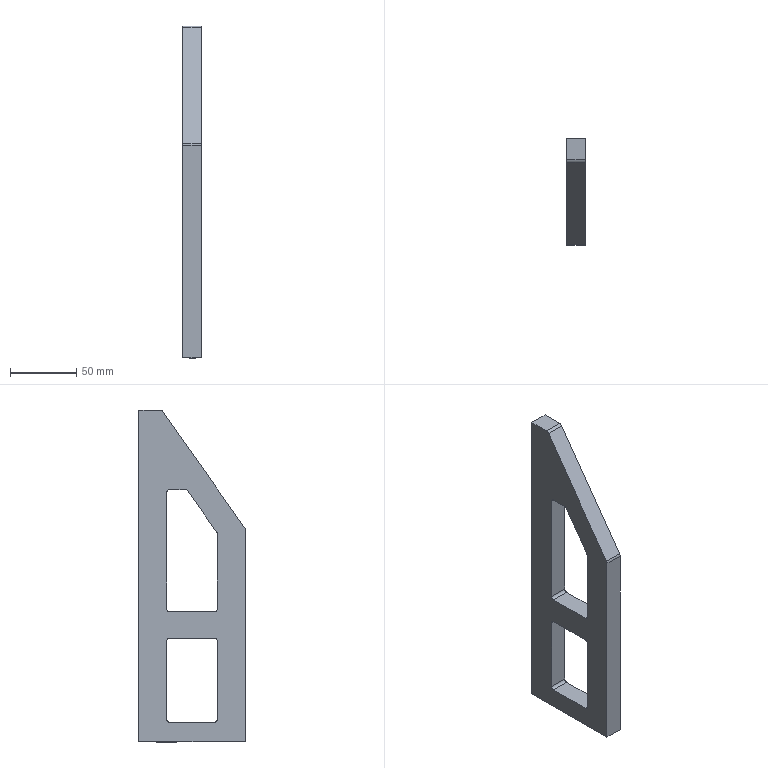Part | SolidWorks | features Fillet 3, Cut 2, HoleWzd 2, Extrusion 1 | 1 solid | 47 faces | box 14 x 80 x 250 mm | volume 162900 mm3 | cylinder 21 | plane 16 | cone 10 | commonest cylinder face diameters 4 x9 3.3 x6 4.2 x4 6 x2
STEP:
#1=CARTESIAN_POINT('',(50.,192.243,112.35));
#2=VERTEX_POINT('',#1);
#3=CARTESIAN_POINT('',(50.,192.243,115.65));
#4=VERTEX_POINT('',#3);
#5=CARTESIAN_POINT('',(50.,192.243,114.));
#6=DIRECTION('',(0.,1.,0.));
#7=DIRECTION('',(0.,0.,1.));
#8=AXIS2_PLACEMENT_3D('',#5,#6,#7);
#9=CIRCLE('',#8,1.65);
#10=EDGE_CURVE('',#2,#4,#9,.T.);
#11=ORIENTED_EDGE('',*,*,#10,.F.);
#12=CARTESIAN_POINT('',(50.,203.743,112.35));
#13=VERTEX_POINT('',#12);
#14=CARTESIAN_POINT('',(50.,203.743,112.35));
#15=DIRECTION('',(0.,1.,0.));
#16=VECTOR('',#15,1000.);
#17=LINE('',#14,#16);
#18=EDGE_CURVE('',#2,#13,#17,.T.);
#19=ORIENTED_EDGE('',*,*,#18,.T.);
#20=CARTESIAN_POINT('',(50.,203.743,115.65));
#21=VERTEX_POINT('',#20);
#22=CARTESIAN_POINT('',(50.,203.743,114.));
#23=DIRECTION('',(0.,1.,0.));
#24=DIRECTION('',(0.,0.,1.));
#25=AXIS2_PLACEMENT_3D('',#22,#23,#24);
#26=CIRCLE('',#25,1.65);
#27=EDGE_CURVE('',#13,#21,#26,.T.);
#28=ORIENTED_EDGE('',*,*,#27,.T.);
#29=CARTESIAN_POINT('',(50.,203.743,115.65));
#30=DIRECTION('',(0.,1.,0.));
#31=VECTOR('',#30,1000.);
#32=LINE('',#29,#31);
#33=EDGE_CURVE('',#4,#21,#32,.T.);
#34=ORIENTED_EDGE('',*,*,#33,.F.);
#35=EDGE_LOOP('',(#11,#19,#28,#34));
#36=FACE_OUTER_BOUND('',#35,.T.);
#37=CARTESIAN_POINT('',(50.,203.743,114.));
#38=DIRECTION('',(0.,1.,0.));
#39=DIRECTION('',(0.,0.,1.));
#40=AXIS2_PLACEMENT_3D('',#37,#38,#39);
#41=CYLINDRICAL_SURFACE('',#40,1.65);
#42=ADVANCED_FACE('',(#36),#41,.F.);
#43=CARTESIAN_POINT('',(50.,191.252,114.));
#44=VERTEX_POINT('',#43);
#45=CARTESIAN_POINT('',(50.,192.243,115.65));
#46=DIRECTION('',(0.,0.515,0.8572));
#47=VECTOR('',#46,1000.);
#48=LINE('',#45,#47);
#49=EDGE_CURVE('',#44,#4,#48,.T.);
#50=ORIENTED_EDGE('',*,*,#49,.F.);
#51=CARTESIAN_POINT('',(50.,192.243,112.35));
#52=DIRECTION('',(0.,0.515,-0.8572));
#53=VECTOR('',#52,1000.);
#54=LINE('',#51,#53);
#55=EDGE_CURVE('',#44,#2,#54,.T.);
#56=ORIENTED_EDGE('',*,*,#55,.T.);
#57=ORIENTED_EDGE('',*,*,#10,.T.);
#58=EDGE_LOOP('',(#50,#56,#57));
#59=FACE_OUTER_BOUND('',#58,.T.);
#60=CARTESIAN_POINT('',(50.,192.243,114.));
#61=DIRECTION('',(0.,1.,0.));
#62=DIRECTION('',(0.,0.,1.));
#63=AXIS2_PLACEMENT_3D('',#60,#61,#62);
#64=CONICAL_SURFACE('',#63,1.65,1.03);
#65=ADVANCED_FACE('',(#59),#64,.F.);
#66=CARTESIAN_POINT('',(50.,192.243,172.35));
#67=VERTEX_POINT('',#66);
#68=CARTESIAN_POINT('',(50.,192.243,175.65));
#69=VERTEX_POINT('',#68);
#70=CARTESIAN_POINT('',(50.,192.243,174.));
#71=DIRECTION('',(0.,1.,0.));
#72=DIRECTION('',(0.,0.,1.));
#73=AXIS2_PLACEMENT_3D('',#70,#71,#72);
#74=CIRCLE('',#73,1.65);
#75=EDGE_CURVE('',#67,#69,#74,.T.);
#76=ORIENTED_EDGE('',*,*,#75,.F.);
#77=CARTESIAN_POINT('',(50.,203.743,172.35));
#78=VERTEX_POINT('',#77);
#79=CARTESIAN_POINT('',(50.,203.743,172.35));
#80=DIRECTION('',(0.,1.,0.));
#81=VECTOR('',#80,1000.);
#82=LINE('',#79,#81);
#83=EDGE_CURVE('',#67,#78,#82,.T.);
#84=ORIENTED_EDGE('',*,*,#83,.T.);
#85=CARTESIAN_POINT('',(50.,203.743,175.65));
#86=VERTEX_POINT('',#85);
#87=CARTESIAN_POINT('',(50.,203.743,174.));
#88=DIRECTION('',(0.,1.,0.));
#89=DIRECTION('',(0.,0.,1.));
#90=AXIS2_PLACEMENT_3D('',#87,#88,#89);
#91=CIRCLE('',#90,1.65);
#92=EDGE_CURVE('',#78,#86,#91,.T.);
#93=ORIENTED_EDGE('',*,*,#92,.T.);
#94=CARTESIAN_POINT('',(50.,203.743,175.65));
#95=DIRECTION('',(0.,1.,0.));
#96=VECTOR('',#95,1000.);
#97=LINE('',#94,#96);
#98=EDGE_CURVE('',#69,#86,#97,.T.);
#99=ORIENTED_EDGE('',*,*,#98,.F.);
#100=EDGE_LOOP('',(#76,#84,#93,#99));
#101=FACE_OUTER_BOUND('',#100,.T.);
#102=CARTESIAN_POINT('',(50.,203.743,174.));
#103=DIRECTION('',(0.,1.,0.));
#104=DIRECTION('',(0.,0.,1.));
#105=AXIS2_PLACEMENT_3D('',#102,#103,#104);
#106=CYLINDRICAL_SURFACE('',#105,1.65);
#107=ADVANCED_FACE('',(#101),#106,.F.);
#108=CARTESIAN_POINT('',(50.,191.252,174.));
#109=VERTEX_POINT('',#108);
#110=CARTESIAN_POINT('',(50.,192.243,175.65));
#111=DIRECTION('',(0.,0.515,0.8572));
#112=VECTOR('',#111,1000.);
#113=LINE('',#110,#112);
#114=EDGE_CURVE('',#109,#69,#113,.T.);
#115=ORIENTED_EDGE('',*,*,#114,.F.);
#116=CARTESIAN_POINT('',(50.,192.243,172.35));
#117=DIRECTION('',(0.,0.515,-0.8572));
#118=VECTOR('',#117,1000.);
#119=LINE('',#116,#118);
#120=EDGE_CURVE('',#109,#67,#119,.T.);
#121=ORIENTED_EDGE('',*,*,#120,.T.);
#122=ORIENTED_EDGE('',*,*,#75,.T.);
#123=EDGE_LOOP('',(#115,#121,#122));
#124=FACE_OUTER_BOUND('',#123,.T.);
#125=CARTESIAN_POINT('',(50.,192.243,174.));
#126=DIRECTION('',(0.,1.,0.));
#127=DIRECTION('',(0.,0.,1.));
#128=AXIS2_PLACEMENT_3D('',#125,#126,#127);
#129=CONICAL_SURFACE('',#128,1.65,1.03);
#130=ADVANCED_FACE('',(#124),#129,.F.);
#131=CARTESIAN_POINT('',(50.,192.243,232.35));
#132=VERTEX_POINT('',#131);
#133=CARTESIAN_POINT('',(50.,192.243,235.65));
#134=VERTEX_POINT('',#133);
#135=CARTESIAN_POINT('',(50.,192.243,234.));
#136=DIRECTION('',(0.,1.,0.));
#137=DIRECTION('',(0.,0.,1.));
#138=AXIS2_PLACEMENT_3D('',#135,#136,#137);
#139=CIRCLE('',#138,1.65);
#140=EDGE_CURVE('',#132,#134,#139,.T.);
#141=ORIENTED_EDGE('',*,*,#140,.F.);
#142=CARTESIAN_POINT('',(50.,203.743,232.35));
#143=VERTEX_POINT('',#142);
#144=CARTESIAN_POINT('',(50.,203.743,232.35));
#145=DIRECTION('',(0.,1.,0.));
#146=VECTOR('',#145,1000.);
#147=LINE('',#144,#146);
#148=EDGE_CURVE('',#132,#143,#147,.T.);
#149=ORIENTED_EDGE('',*,*,#148,.T.);
#150=CARTESIAN_POINT('',(50.,203.743,235.65));
#151=VERTEX_POINT('',#150);
#152=CARTESIAN_POINT('',(50.,203.743,234.));
#153=DIRECTION('',(0.,1.,0.));
#154=DIRECTION('',(0.,0.,1.));
#155=AXIS2_PLACEMENT_3D('',#152,#153,#154);
#156=CIRCLE('',#155,1.65);
#157=EDGE_CURVE('',#143,#151,#156,.T.);
#158=ORIENTED_EDGE('',*,*,#157,.T.);
#159=CARTESIAN_POINT('',(50.,203.743,235.65));
#160=DIRECTION('',(0.,1.,0.));
#161=VECTOR('',#160,1000.);
#162=LINE('',#159,#161);
#163=EDGE_CURVE('',#134,#151,#162,.T.);
#164=ORIENTED_EDGE('',*,*,#163,.F.);
#165=EDGE_LOOP('',(#141,#149,#158,#164));
#166=FACE_OUTER_BOUND('',#165,.T.);
#167=CARTESIAN_POINT('',(50.,203.743,234.));
#168=DIRECTION('',(0.,1.,0.));
#169=DIRECTION('',(0.,0.,1.));
#170=AXIS2_PLACEMENT_3D('',#167,#168,#169);
#171=CYLINDRICAL_SURFACE('',#170,1.65);
#172=ADVANCED_FACE('',(#166),#171,.F.);
#173=CARTESIAN_POINT('',(50.,191.252,234.));
#174=VERTEX_POINT('',#173);
#175=CARTESIAN_POINT('',(50.,192.243,235.65));
#176=DIRECTION('',(0.,0.515,0.8572));
#177=VECTOR('',#176,1000.);
#178=LINE('',#175,#177);
#179=EDGE_CURVE('',#174,#134,#178,.T.);
#180=ORIENTED_EDGE('',*,*,#179,.F.);
#181=CARTESIAN_POINT('',(50.,192.243,232.35));
#182=DIRECTION('',(0.,0.515,-0.8572));
#183=VECTOR('',#182,1000.);
#184=LINE('',#181,#183);
#185=EDGE_CURVE('',#174,#132,#184,.T.);
#186=ORIENTED_EDGE('',*,*,#185,.T.);
#187=ORIENTED_EDGE('',*,*,#140,.T.);
#188=EDGE_LOOP('',(#180,#186,#187));
#189=FACE_OUTER_BOUND('',#188,.T.);
#190=CARTESIAN_POINT('',(50.,192.243,234.));
#191=DIRECTION('',(0.,1.,0.));
#192=DIRECTION('',(0.,0.,1.));
#193=AXIS2_PLACEMENT_3D('',#190,#191,#192);
#194=CONICAL_SURFACE('',#193,1.65,1.03);
#195=ADVANCED_FACE('',(#189),#194,.F.);
#196=CARTESIAN_POINT('',(50.5,186.643,14.));
#197=VERTEX_POINT('',#196);
#198=CARTESIAN_POINT('',(50.5,190.843,14.));
#199=VERTEX_POINT('',#198);
#200=CARTESIAN_POINT('',(50.5,188.743,14.));
#201=DIRECTION('',(0.,0.,-1.));
#202=DIRECTION('',(0.,1.,0.));
#203=AXIS2_PLACEMENT_3D('',#200,#201,#202);
#204=CIRCLE('',#203,2.1);
#205=EDGE_CURVE('',#197,#199,#204,.T.);
#206=ORIENTED_EDGE('',*,*,#205,.F.);
#207=CARTESIAN_POINT('',(50.5,186.643,0.));
#208=VERTEX_POINT('',#207);
#209=CARTESIAN_POINT('',(50.5,186.643,0.));
#210=DIRECTION('',(0.,0.,-1.));
#211=VECTOR('',#210,1000.);
#212=LINE('',#209,#211);
#213=EDGE_CURVE('',#197,#208,#212,.T.);
#214=ORIENTED_EDGE('',*,*,#213,.T.);
#215=CARTESIAN_POINT('',(50.5,190.843,0.));
#216=VERTEX_POINT('',#215);
#217=CARTESIAN_POINT('',(50.5,188.743,0.));
#218=DIRECTION('',(0.,0.,-1.));
#219=DIRECTION('',(0.,1.,0.));
#220=AXIS2_PLACEMENT_3D('',#217,#218,#219);
#221=CIRCLE('',#220,2.1);
#222=EDGE_CURVE('',#208,#216,#221,.T.);
#223=ORIENTED_EDGE('',*,*,#222,.T.);
#224=CARTESIAN_POINT('',(50.5,190.843,0.));
#225=DIRECTION('',(0.,0.,-1.));
#226=VECTOR('',#225,1000.);
#227=LINE('',#224,#226);
#228=EDGE_CURVE('',#199,#216,#227,.T.);
#229=ORIENTED_EDGE('',*,*,#228,.F.);
#230=EDGE_LOOP('',(#206,#214,#223,#229));
#231=FACE_OUTER_BOUND('',#230,.T.);
#232=CARTESIAN_POINT('',(50.5,188.743,0.));
#233=DIRECTION('',(0.,0.,-1.));
#234=DIRECTION('',(0.,1.,0.));
#235=AXIS2_PLACEMENT_3D('',#232,#233,#234);
#236=CYLINDRICAL_SURFACE('',#235,2.1);
#237=ADVANCED_FACE('',(#231),#236,.F.);
#238=CARTESIAN_POINT('',(50.5,188.743,15.262));
#239=VERTEX_POINT('',#238);
#240=CARTESIAN_POINT('',(50.5,190.843,14.));
#241=DIRECTION('',(0.,0.8572,-0.515));
#242=VECTOR('',#241,1000.);
#243=LINE('',#240,#242);
#244=EDGE_CURVE('',#239,#199,#243,.T.);
#245=ORIENTED_EDGE('',*,*,#244,.F.);
#246=CARTESIAN_POINT('',(50.5,186.643,14.));
#247=DIRECTION('',(0.,-0.8572,-0.515));
#248=VECTOR('',#247,1000.);
#249=LINE('',#246,#248);
#250=EDGE_CURVE('',#239,#197,#249,.T.);
#251=ORIENTED_EDGE('',*,*,#250,.T.);
#252=ORIENTED_EDGE('',*,*,#205,.T.);
#253=EDGE_LOOP('',(#245,#251,#252));
#254=FACE_OUTER_BOUND('',#253,.T.);
#255=CARTESIAN_POINT('',(50.5,188.743,14.));
#256=DIRECTION('',(0.,0.,-1.));
#257=DIRECTION('',(0.,1.,0.));
#258=AXIS2_PLACEMENT_3D('',#255,#256,#257);
#259=CONICAL_SURFACE('',#258,2.1,1.03);
#260=ADVANCED_FACE('',(#254),#259,.F.);
#261=CARTESIAN_POINT('',(50.,136.645,14.));
#262=VERTEX_POINT('',#261);
#263=CARTESIAN_POINT('',(50.,140.845,14.));
#264=VERTEX_POINT('',#263);
#265=CARTESIAN_POINT('',(50.,138.745,14.));
#266=DIRECTION('',(0.,0.,-1.));
#267=DIRECTION('',(0.,1.,0.));
#268=AXIS2_PLACEMENT_3D('',#265,#266,#267);
#269=CIRCLE('',#268,2.1);
#270=EDGE_CURVE('',#262,#264,#269,.T.);
#271=ORIENTED_EDGE('',*,*,#270,.F.);
#272=CARTESIAN_POINT('',(50.,136.645,0.));
#273=VERTEX_POINT('',#272);
#274=CARTESIAN_POINT('',(50.,136.645,0.));
#275=DIRECTION('',(0.,0.,-1.));
#276=VECTOR('',#275,1000.);
#277=LINE('',#274,#276);
#278=EDGE_CURVE('',#262,#273,#277,.T.);
#279=ORIENTED_EDGE('',*,*,#278,.T.);
#280=CARTESIAN_POINT('',(50.,140.845,0.));
#281=VERTEX_POINT('',#280);
#282=CARTESIAN_POINT('',(50.,138.745,0.));
#283=DIRECTION('',(0.,0.,-1.));
#284=DIRECTION('',(0.,1.,0.));
#285=AXIS2_PLACEMENT_3D('',#282,#283,#284);
#286=CIRCLE('',#285,2.1);
#287=EDGE_CURVE('',#273,#281,#286,.T.);
#288=ORIENTED_EDGE('',*,*,#287,.T.);
#289=CARTESIAN_POINT('',(50.,140.845,0.));
#290=DIRECTION('',(0.,0.,-1.));
#291=VECTOR('',#290,1000.);
#292=LINE('',#289,#291);
#293=EDGE_CURVE('',#264,#281,#292,.T.);
#294=ORIENTED_EDGE('',*,*,#293,.F.);
#295=EDGE_LOOP('',(#271,#279,#288,#294));
#296=FACE_OUTER_BOUND('',#295,.T.);
#297=CARTESIAN_POINT('',(50.,138.745,0.));
#298=DIRECTION('',(0.,0.,-1.));
#299=DIRECTION('',(0.,1.,0.));
#300=AXIS2_PLACEMENT_3D('',#297,#298,#299);
#301=CYLINDRICAL_SURFACE('',#300,2.1);
#302=ADVANCED_FACE('',(#296),#301,.F.);
#303=CARTESIAN_POINT('',(50.,138.745,15.262));
#304=VERTEX_POINT('',#303);
#305=CARTESIAN_POINT('',(50.,140.845,14.));
#306=DIRECTION('',(0.,0.8572,-0.515));
#307=VECTOR('',#306,1000.);
#308=LINE('',#305,#307);
#309=EDGE_CURVE('',#304,#264,#308,.T.);
#310=ORIENTED_EDGE('',*,*,#309,.F.);
#311=CARTESIAN_POINT('',(50.,136.645,14.));
#312=DIRECTION('',(0.,-0.8572,-0.515));
#313=VECTOR('',#312,1000.);
#314=LINE('',#311,#313);
#315=EDGE_CURVE('',#304,#262,#314,.T.);
#316=ORIENTED_EDGE('',*,*,#315,.T.);
#317=ORIENTED_EDGE('',*,*,#270,.T.);
#318=EDGE_LOOP('',(#310,#316,#317));
#319=FACE_OUTER_BOUND('',#318,.T.);
#320=CARTESIAN_POINT('',(50.,138.745,14.));
#321=DIRECTION('',(0.,0.,-1.));
#322=DIRECTION('',(0.,1.,0.));
#323=AXIS2_PLACEMENT_3D('',#320,#321,#322);
#324=CONICAL_SURFACE('',#323,2.1,1.03);
#325=ADVANCED_FACE('',(#319),#324,.F.);
#326=CARTESIAN_POINT('',(50.,203.743,114.));
#327=DIRECTION('',(0.,1.,0.));
#328=DIRECTION('',(0.,0.,1.));
#329=AXIS2_PLACEMENT_3D('',#326,#327,#328);
#330=CIRCLE('',#329,1.65);
#331=EDGE_CURVE('',#21,#13,#330,.T.);
#332=ORIENTED_EDGE('',*,*,#331,.F.);
#333=ORIENTED_EDGE('',*,*,#27,.F.);
#334=EDGE_LOOP('',(#332,#333));
#335=FACE_BOUND('',#334,.T.);
#336=CARTESIAN_POINT('',(50.,203.743,174.));
#337=DIRECTION('',(0.,1.,0.));
#338=DIRECTION('',(0.,0.,1.));
#339=AXIS2_PLACEMENT_3D('',#336,#337,#338);
#340=CIRCLE('',#339,1.65);
#341=EDGE_CURVE('',#86,#78,#340,.T.);
#342=ORIENTED_EDGE('',*,*,#341,.F.);
#343=ORIENTED_EDGE('',*,*,#92,.F.);
#344=EDGE_LOOP('',(#342,#343));
#345=FACE_BOUND('',#344,.T.);
#346=CARTESIAN_POINT('',(50.,203.743,234.));
#347=DIRECTION('',(0.,1.,0.));
#348=DIRECTION('',(0.,0.,1.));
#349=AXIS2_PLACEMENT_3D('',#346,#347,#348);
#350=CIRCLE('',#349,1.65);
#351=EDGE_CURVE('',#151,#143,#350,.T.);
#352=ORIENTED_EDGE('',*,*,#351,.F.);
#353=ORIENTED_EDGE('',*,*,#157,.F.);
#354=EDGE_LOOP('',(#352,#353));
#355=FACE_BOUND('',#354,.T.);
#356=CARTESIAN_POINT('',(57.,203.743,250.));
#357=VERTEX_POINT('',#356);
#358=CARTESIAN_POINT('',(57.,203.743,0.));
#359=VERTEX_POINT('',#358);
#360=CARTESIAN_POINT('',(57.,203.743,250.));
#361=DIRECTION('',(0.,0.,-1.));
#362=VECTOR('',#361,1000.);
#363=LINE('',#360,#362);
#364=EDGE_CURVE('',#357,#359,#363,.T.);
#365=ORIENTED_EDGE('',*,*,#364,.T.);
#366=CARTESIAN_POINT('',(43.,203.743,0.));
#367=VERTEX_POINT('',#366);
#368=CARTESIAN_POINT('',(43.,203.743,0.));
#369=DIRECTION('',(1.,0.,0.));
#370=VECTOR('',#369,1000.);
#371=LINE('',#368,#370);
#372=EDGE_CURVE('',#367,#359,#371,.T.);
#373=ORIENTED_EDGE('',*,*,#372,.F.);
#374=CARTESIAN_POINT('',(43.,203.743,250.));
#375=VERTEX_POINT('',#374);
#376=CARTESIAN_POINT('',(43.,203.743,250.));
#377=DIRECTION('',(0.,0.,-1.));
#378=VECTOR('',#377,1000.);
#379=LINE('',#376,#378);
#380=EDGE_CURVE('',#375,#367,#379,.T.);
#381=ORIENTED_EDGE('',*,*,#380,.F.);
#382=CARTESIAN_POINT('',(43.,203.743,250.));
#383=DIRECTION('',(1.,0.,0.));
#384=VECTOR('',#383,1000.);
#385=LINE('',#382,#384);
#386=EDGE_CURVE('',#375,#357,#385,.T.);
#387=ORIENTED_EDGE('',*,*,#386,.T.);
#388=EDGE_LOOP('',(#365,#373,#381,#387));
#389=FACE_OUTER_BOUND('',#388,.T.);
#390=CARTESIAN_POINT('',(43.,203.743,250.));
#391=DIRECTION('',(0.,-1.,0.));
#392=DIRECTION('',(1.,0.,0.));
#393=AXIS2_PLACEMENT_3D('',#390,#391,#392);
#394=PLANE('',#393);
#395=ADVANCED_FACE('',(#335,#345,#355,#389),#394,.F.);
#396=CARTESIAN_POINT('',(50.5,188.743,0.));
#397=DIRECTION('',(0.,0.,-1.));
#398=DIRECTION('',(0.,1.,0.));
#399=AXIS2_PLACEMENT_3D('',#396,#397,#398);
#400=CIRCLE('',#399,2.1);
#401=EDGE_CURVE('',#216,#208,#400,.T.);
#402=ORIENTED_EDGE('',*,*,#401,.F.);
#403=ORIENTED_EDGE('',*,*,#222,.F.);
#404=EDGE_LOOP('',(#402,#403));
#405=FACE_BOUND('',#404,.T.);
#406=CARTESIAN_POINT('',(50.,138.745,0.));
#407=DIRECTION('',(0.,0.,-1.));
#408=DIRECTION('',(0.,1.,0.));
#409=AXIS2_PLACEMENT_3D('',#406,#407,#408);
#410=CIRCLE('',#409,2.1);
#411=EDGE_CURVE('',#281,#273,#410,.T.);
#412=ORIENTED_EDGE('',*,*,#411,.F.);
#413=ORIENTED_EDGE('',*,*,#287,.F.);
#414=EDGE_LOOP('',(#412,#413));
#415=FACE_BOUND('',#414,.T.);
#416=CARTESIAN_POINT('',(57.,123.743,0.));
#417=VERTEX_POINT('',#416);
#418=CARTESIAN_POINT('',(57.,203.743,0.));
#419=DIRECTION('',(0.,-1.,0.));
#420=VECTOR('',#419,1000.);
#421=LINE('',#418,#420);
#422=EDGE_CURVE('',#359,#417,#421,.T.);
#423=ORIENTED_EDGE('',*,*,#422,.T.);
#424=CARTESIAN_POINT('',(43.,123.743,0.));
#425=VERTEX_POINT('',#424);
#426=CARTESIAN_POINT('',(43.,123.743,0.));
#427=DIRECTION('',(1.,0.,0.));
#428=VECTOR('',#427,1000.);
#429=LINE('',#426,#428);
#430=EDGE_CURVE('',#425,#417,#429,.T.);
#431=ORIENTED_EDGE('',*,*,#430,.F.);
#432=CARTESIAN_POINT('',(43.,203.743,0.));
#433=DIRECTION('',(0.,-1.,0.));
#434=VECTOR('',#433,1000.);
#435=LINE('',#432,#434);
#436=EDGE_CURVE('',#367,#425,#435,.T.);
#437=ORIENTED_EDGE('',*,*,#436,.F.);
#438=ORIENTED_EDGE('',*,*,#372,.T.);
#439=EDGE_LOOP('',(#423,#431,#437,#438));
#440=FACE_OUTER_BOUND('',#439,.T.);
#441=CARTESIAN_POINT('',(43.,203.743,0.));
#442=DIRECTION('',(0.,0.,1.));
#443=DIRECTION('',(0.,-1.,0.));
#444=AXIS2_PLACEMENT_3D('',#441,#442,#443);
#445=PLANE('',#444);
#446=ADVANCED_FACE('',(#405,#415,#440),#445,.F.);
#447=CARTESIAN_POINT('',(57.,123.743,160.046));
#448=VERTEX_POINT('',#447);
#449=CARTESIAN_POINT('',(57.,123.743,0.));
#450=DIRECTION('',(0.,0.,1.));
#451=VECTOR('',#450,1000.);
#452=LINE('',#449,#451);
#453=EDGE_CURVE('',#417,#448,#452,.T.);
#454=ORIENTED_EDGE('',*,*,#453,.T.);
#455=CARTESIAN_POINT('',(43.,123.743,160.046));
#456=VERTEX_POINT('',#455);
#457=CARTESIAN_POINT('',(43.,123.743,160.046));
#458=DIRECTION('',(-1.,0.,0.));
#459=VECTOR('',#458,1000.);
#460=LINE('',#457,#459);
#461=EDGE_CURVE('',#448,#456,#460,.T.);
#462=ORIENTED_EDGE('',*,*,#461,.T.);
#463=CARTESIAN_POINT('',(43.,123.743,0.));
#464=DIRECTION('',(0.,0.,1.));
#465=VECTOR('',#464,1000.);
#466=LINE('',#463,#465);
#467=EDGE_CURVE('',#425,#456,#466,.T.);
#468=ORIENTED_EDGE('',*,*,#467,.F.);
#469=ORIENTED_EDGE('',*,*,#430,.T.);
#470=EDGE_LOOP('',(#454,#462,#468,#469));
#471=FACE_OUTER_BOUND('',#470,.T.);
#472=CARTESIAN_POINT('',(43.,123.743,0.));
#473=DIRECTION('',(0.,1.,0.));
#474=DIRECTION('',(0.,0.,1.));
#475=AXIS2_PLACEMENT_3D('',#472,#473,#474);
#476=PLANE('',#475);
#477=ADVANCED_FACE('',(#471),#476,.F.);
#478=CARTESIAN_POINT('',(57.,124.294,161.779));
#479=VERTEX_POINT('',#478);
#480=CARTESIAN_POINT('',(57.,185.846,248.733));
#481=VERTEX_POINT('',#480);
#482=CARTESIAN_POINT('',(57.,123.743,161.));
#483=DIRECTION('',(0.,0.5778,0.8162));
#484=VECTOR('',#483,1000.);
#485=LINE('',#482,#484);
#486=EDGE_CURVE('',#479,#481,#485,.T.);
#487=ORIENTED_EDGE('',*,*,#486,.T.);
#488=CARTESIAN_POINT('',(43.,185.846,248.733));
#489=VERTEX_POINT('',#488);
#490=CARTESIAN_POINT('',(43.,185.846,248.733));
#491=DIRECTION('',(-1.,0.,0.));
#492=VECTOR('',#491,1000.);
#493=LINE('',#490,#492);
#494=EDGE_CURVE('',#481,#489,#493,.T.);
#495=ORIENTED_EDGE('',*,*,#494,.T.);
#496=CARTESIAN_POINT('',(43.,124.294,161.779));
#497=VERTEX_POINT('',#496);
#498=CARTESIAN_POINT('',(43.,123.743,161.));
#499=DIRECTION('',(0.,0.5778,0.8162));
#500=VECTOR('',#499,1000.);
#501=LINE('',#498,#500);
#502=EDGE_CURVE('',#497,#489,#501,.T.);
#503=ORIENTED_EDGE('',*,*,#502,.F.);
#504=CARTESIAN_POINT('',(43.,124.294,161.779));
#505=DIRECTION('',(1.,0.,0.));
#506=VECTOR('',#505,1000.);
#507=LINE('',#504,#506);
#508=EDGE_CURVE('',#497,#479,#507,.T.);
#509=ORIENTED_EDGE('',*,*,#508,.T.);
#510=EDGE_LOOP('',(#487,#495,#503,#509));
#511=FACE_OUTER_BOUND('',#510,.T.);
#512=CARTESIAN_POINT('',(43.,123.743,161.));
#513=DIRECTION('',(0.,0.8162,-0.5778));
#514=DIRECTION('',(0.,0.5778,0.8162));
#515=AXIS2_PLACEMENT_3D('',#512,#513,#514);
#516=PLANE('',#515);
#517=ADVANCED_FACE('',(#511),#516,.F.);
#518=CARTESIAN_POINT('',(43.,188.295,250.));
#519=VERTEX_POINT('',#518);
#520=CARTESIAN_POINT('',(43.,186.743,250.));
#521=DIRECTION('',(0.,1.,0.));
#522=VECTOR('',#521,1000.);
#523=LINE('',#520,#522);
#524=EDGE_CURVE('',#519,#375,#523,.T.);
#525=ORIENTED_EDGE('',*,*,#524,.F.);
#526=CARTESIAN_POINT('',(57.,188.295,250.));
#527=VERTEX_POINT('',#526);
#528=CARTESIAN_POINT('',(43.,188.295,250.));
#529=DIRECTION('',(1.,0.,0.));
#530=VECTOR('',#529,1000.);
#531=LINE('',#528,#530);
#532=EDGE_CURVE('',#519,#527,#531,.T.);
#533=ORIENTED_EDGE('',*,*,#532,.T.);
#534=CARTESIAN_POINT('',(57.,186.743,250.));
#535=DIRECTION('',(0.,1.,0.));
#536=VECTOR('',#535,1000.);
#537=LINE('',#534,#536);
#538=EDGE_CURVE('',#527,#357,#537,.T.);
#539=ORIENTED_EDGE('',*,*,#538,.T.);
#540=ORIENTED_EDGE('',*,*,#386,.F.);
#541=EDGE_LOOP('',(#525,#533,#539,#540));
#542=FACE_OUTER_BOUND('',#541,.T.);
#543=CARTESIAN_POINT('',(43.,186.743,250.));
#544=DIRECTION('',(0.,0.,-1.));
#545=DIRECTION('',(-1.,0.,0.));
#546=AXIS2_PLACEMENT_3D('',#543,#544,#545);
#547=PLANE('',#546);
#548=ADVANCED_FACE('',(#542),#547,.F.);
#549=CARTESIAN_POINT('',(43.,144.743,156.872));
#550=VERTEX_POINT('',#549);
#551=CARTESIAN_POINT('',(43.,144.743,100.));
#552=VERTEX_POINT('',#551);
#553=CARTESIAN_POINT('',(43.,144.743,98.));
#554=DIRECTION('',(0.,0.,-1.));
#555=VECTOR('',#554,1000.);
#556=LINE('',#553,#555);
#557=EDGE_CURVE('',#550,#552,#556,.T.);
#558=ORIENTED_EDGE('',*,*,#557,.T.);
#559=CARTESIAN_POINT('',(43.,146.743,98.));
#560=VERTEX_POINT('',#559);
#561=CARTESIAN_POINT('',(43.,146.743,100.));
#562=DIRECTION('',(1.,0.,0.));
#563=DIRECTION('',(0.,-1.,0.));
#564=AXIS2_PLACEMENT_3D('',#561,#562,#563);
#565=CIRCLE('',#564,2.);
#566=EDGE_CURVE('',#552,#560,#565,.T.);
#567=ORIENTED_EDGE('',*,*,#566,.T.);
#568=CARTESIAN_POINT('',(43.,180.743,98.));
#569=VERTEX_POINT('',#568);
#570=CARTESIAN_POINT('',(43.,144.743,98.));
#571=DIRECTION('',(0.,1.,0.));
#572=VECTOR('',#571,1000.);
#573=LINE('',#570,#572);
#574=EDGE_CURVE('',#560,#569,#573,.T.);
#575=ORIENTED_EDGE('',*,*,#574,.T.);
#576=CARTESIAN_POINT('',(43.,182.743,100.));
#577=VERTEX_POINT('',#576);
#578=CARTESIAN_POINT('',(43.,180.743,100.));
#579=DIRECTION('',(1.,0.,0.));
#580=DIRECTION('',(0.,-1.,0.));
#581=AXIS2_PLACEMENT_3D('',#578,#579,#580);
#582=CIRCLE('',#581,2.);
#583=EDGE_CURVE('',#569,#577,#582,.T.);
#584=ORIENTED_EDGE('',*,*,#583,.T.);
#585=CARTESIAN_POINT('',(43.,182.743,188.));
#586=VERTEX_POINT('',#585);
#587=CARTESIAN_POINT('',(43.,182.743,98.));
#588=DIRECTION('',(0.,0.,1.));
#589=VECTOR('',#588,1000.);
#590=LINE('',#587,#589);
#591=EDGE_CURVE('',#577,#586,#590,.T.);
#592=ORIENTED_EDGE('',*,*,#591,.T.);
#593=CARTESIAN_POINT('',(43.,180.743,190.));
#594=VERTEX_POINT('',#593);
#595=CARTESIAN_POINT('',(43.,180.743,188.));
#596=DIRECTION('',(1.,0.,0.));
#597=DIRECTION('',(0.,-1.,0.));
#598=AXIS2_PLACEMENT_3D('',#595,#596,#597);
#599=CIRCLE('',#598,2.);
#600=EDGE_CURVE('',#586,#594,#599,.T.);
#601=ORIENTED_EDGE('',*,*,#600,.T.);
#602=CARTESIAN_POINT('',(43.,168.778,190.));
#603=VERTEX_POINT('',#602);
#604=CARTESIAN_POINT('',(43.,167.743,190.));
#605=DIRECTION('',(0.,-1.,0.));
#606=VECTOR('',#605,1000.);
#607=LINE('',#604,#606);
#608=EDGE_CURVE('',#594,#603,#607,.T.);
#609=ORIENTED_EDGE('',*,*,#608,.T.);
#610=CARTESIAN_POINT('',(43.,167.145,189.156));
#611=VERTEX_POINT('',#610);
#612=CARTESIAN_POINT('',(43.,168.778,188.));
#613=DIRECTION('',(1.,0.,0.));
#614=DIRECTION('',(0.,-1.,0.));
#615=AXIS2_PLACEMENT_3D('',#612,#613,#614);
#616=CIRCLE('',#615,2.);
#617=EDGE_CURVE('',#603,#611,#616,.T.);
#618=ORIENTED_EDGE('',*,*,#617,.T.);
#619=CARTESIAN_POINT('',(43.,145.111,158.027));
#620=VERTEX_POINT('',#619);
#621=CARTESIAN_POINT('',(43.,144.743,157.508));
#622=DIRECTION('',(0.,-0.5778,-0.8162));
#623=VECTOR('',#622,1000.);
#624=LINE('',#621,#623);
#625=EDGE_CURVE('',#611,#620,#624,.T.);
#626=ORIENTED_EDGE('',*,*,#625,.T.);
#627=CARTESIAN_POINT('',(43.,146.743,156.872));
#628=DIRECTION('',(1.,0.,0.));
#629=DIRECTION('',(0.,-1.,0.));
#630=AXIS2_PLACEMENT_3D('',#627,#628,#629);
#631=CIRCLE('',#630,2.);
#632=EDGE_CURVE('',#620,#550,#631,.T.);
#633=ORIENTED_EDGE('',*,*,#632,.T.);
#634=EDGE_LOOP('',(#558,#567,#575,#584,#592,#601,#609,#618,#626,#633));
#635=FACE_BOUND('',#634,.T.);
#636=CARTESIAN_POINT('',(43.,144.743,76.));
#637=VERTEX_POINT('',#636);
#638=CARTESIAN_POINT('',(43.,144.743,17.));
#639=VERTEX_POINT('',#638);
#640=CARTESIAN_POINT('',(43.,144.743,15.));
#641=DIRECTION('',(0.,0.,-1.));
#642=VECTOR('',#641,1000.);
#643=LINE('',#640,#642);
#644=EDGE_CURVE('',#637,#639,#643,.T.);
#645=ORIENTED_EDGE('',*,*,#644,.T.);
#646=CARTESIAN_POINT('',(43.,146.743,15.));
#647=VERTEX_POINT('',#646);
#648=CARTESIAN_POINT('',(43.,146.743,17.));
#649=DIRECTION('',(1.,0.,0.));
#650=DIRECTION('',(0.,-1.,0.));
#651=AXIS2_PLACEMENT_3D('',#648,#649,#650);
#652=CIRCLE('',#651,2.);
#653=EDGE_CURVE('',#639,#647,#652,.T.);
#654=ORIENTED_EDGE('',*,*,#653,.T.);
#655=CARTESIAN_POINT('',(43.,180.743,15.));
#656=VERTEX_POINT('',#655);
#657=CARTESIAN_POINT('',(43.,182.743,15.));
#658=DIRECTION('',(0.,1.,0.));
#659=VECTOR('',#658,1000.);
#660=LINE('',#657,#659);
#661=EDGE_CURVE('',#647,#656,#660,.T.);
#662=ORIENTED_EDGE('',*,*,#661,.T.);
#663=CARTESIAN_POINT('',(43.,182.743,17.));
#664=VERTEX_POINT('',#663);
#665=CARTESIAN_POINT('',(43.,180.743,17.));
#666=DIRECTION('',(1.,0.,0.));
#667=DIRECTION('',(0.,-1.,0.));
#668=AXIS2_PLACEMENT_3D('',#665,#666,#667);
#669=CIRCLE('',#668,2.);
#670=EDGE_CURVE('',#656,#664,#669,.T.);
#671=ORIENTED_EDGE('',*,*,#670,.T.);
#672=CARTESIAN_POINT('',(43.,182.743,76.));
#673=VERTEX_POINT('',#672);
#674=CARTESIAN_POINT('',(43.,182.743,15.));
#675=DIRECTION('',(0.,0.,1.));
#676=VECTOR('',#675,1000.);
#677=LINE('',#674,#676);
#678=EDGE_CURVE('',#664,#673,#677,.T.);
#679=ORIENTED_EDGE('',*,*,#678,.T.);
#680=CARTESIAN_POINT('',(43.,180.743,78.));
#681=VERTEX_POINT('',#680);
#682=CARTESIAN_POINT('',(43.,180.743,76.));
#683=DIRECTION('',(1.,0.,0.));
#684=DIRECTION('',(0.,-1.,0.));
#685=AXIS2_PLACEMENT_3D('',#682,#683,#684);
#686=CIRCLE('',#685,2.);
#687=EDGE_CURVE('',#673,#681,#686,.T.);
#688=ORIENTED_EDGE('',*,*,#687,.T.);
#689=CARTESIAN_POINT('',(43.,146.743,78.));
#690=VERTEX_POINT('',#689);
#691=CARTESIAN_POINT('',(43.,182.743,78.));
#692=DIRECTION('',(0.,-1.,0.));
#693=VECTOR('',#692,1000.);
#694=LINE('',#691,#693);
#695=EDGE_CURVE('',#681,#690,#694,.T.);
#696=ORIENTED_EDGE('',*,*,#695,.T.);
#697=CARTESIAN_POINT('',(43.,146.743,76.));
#698=DIRECTION('',(1.,0.,0.));
#699=DIRECTION('',(0.,-1.,0.));
#700=AXIS2_PLACEMENT_3D('',#697,#698,#699);
#701=CIRCLE('',#700,2.);
#702=EDGE_CURVE('',#690,#637,#701,.T.);
#703=ORIENTED_EDGE('',*,*,#702,.T.);
#704=EDGE_LOOP('',(#645,#654,#662,#671,#679,#688,#696,#703));
#705=FACE_BOUND('',#704,.T.);
#706=ORIENTED_EDGE('',*,*,#502,.T.);
#707=CARTESIAN_POINT('',(43.,188.295,247.));
#708=DIRECTION('',(-1.,0.,0.));
#709=DIRECTION('',(0.,-1.,0.));
#710=AXIS2_PLACEMENT_3D('',#707,#708,#709);
#711=CIRCLE('',#710,3.);
#712=EDGE_CURVE('',#489,#519,#711,.T.);
#713=ORIENTED_EDGE('',*,*,#712,.T.);
#714=ORIENTED_EDGE('',*,*,#524,.T.);
#715=ORIENTED_EDGE('',*,*,#380,.T.);
#716=ORIENTED_EDGE('',*,*,#436,.T.);
#717=ORIENTED_EDGE('',*,*,#467,.T.);
#718=CARTESIAN_POINT('',(43.,126.743,160.046));
#719=DIRECTION('',(-1.,0.,0.));
#720=DIRECTION('',(0.,-1.,0.));
#721=AXIS2_PLACEMENT_3D('',#718,#719,#720);
#722=CIRCLE('',#721,3.);
#723=EDGE_CURVE('',#456,#497,#722,.T.);
#724=ORIENTED_EDGE('',*,*,#723,.T.);
#725=EDGE_LOOP('',(#706,#713,#714,#715,#716,#717,#724));
#726=FACE_OUTER_BOUND('',#725,.T.);
#727=CARTESIAN_POINT('',(43.,0.,0.));
#728=DIRECTION('',(-1.,0.,0.));
#729=DIRECTION('',(0.,-1.,0.));
#730=AXIS2_PLACEMENT_3D('',#727,#728,#729);
#731=PLANE('',#730);
#732=ADVANCED_FACE('',(#635,#705,#726),#731,.T.);
#733=CARTESIAN_POINT('',(57.,182.743,100.));
#734=VERTEX_POINT('',#733);
#735=CARTESIAN_POINT('',(57.,182.743,188.));
#736=VERTEX_POINT('',#735);
#737=CARTESIAN_POINT('',(57.,182.743,98.));
#738=DIRECTION('',(0.,0.,1.));
#739=VECTOR('',#738,1000.);
#740=LINE('',#737,#739);
#741=EDGE_CURVE('',#734,#736,#740,.T.);
#742=ORIENTED_EDGE('',*,*,#741,.F.);
#743=CARTESIAN_POINT('',(57.,180.743,98.));
#744=VERTEX_POINT('',#743);
#745=CARTESIAN_POINT('',(57.,180.743,100.));
#746=DIRECTION('',(-1.,0.,0.));
#747=DIRECTION('',(0.,-1.,0.));
#748=AXIS2_PLACEMENT_3D('',#745,#746,#747);
#749=CIRCLE('',#748,2.);
#750=EDGE_CURVE('',#734,#744,#749,.T.);
#751=ORIENTED_EDGE('',*,*,#750,.T.);
#752=CARTESIAN_POINT('',(57.,146.743,98.));
#753=VERTEX_POINT('',#752);
#754=CARTESIAN_POINT('',(57.,144.743,98.));
#755=DIRECTION('',(0.,1.,0.));
#756=VECTOR('',#755,1000.);
#757=LINE('',#754,#756);
#758=EDGE_CURVE('',#753,#744,#757,.T.);
#759=ORIENTED_EDGE('',*,*,#758,.F.);
#760=CARTESIAN_POINT('',(57.,144.743,100.));
#761=VERTEX_POINT('',#760);
#762=CARTESIAN_POINT('',(57.,146.743,100.));
#763=DIRECTION('',(-1.,0.,0.));
#764=DIRECTION('',(0.,-1.,0.));
#765=AXIS2_PLACEMENT_3D('',#762,#763,#764);
#766=CIRCLE('',#765,2.);
#767=EDGE_CURVE('',#753,#761,#766,.T.);
#768=ORIENTED_EDGE('',*,*,#767,.T.);
#769=CARTESIAN_POINT('',(57.,144.743,156.872));
#770=VERTEX_POINT('',#769);
#771=CARTESIAN_POINT('',(57.,144.743,98.));
#772=DIRECTION('',(0.,0.,-1.));
#773=VECTOR('',#772,1000.);
#774=LINE('',#771,#773);
#775=EDGE_CURVE('',#770,#761,#774,.T.);
#776=ORIENTED_EDGE('',*,*,#775,.F.);
#777=CARTESIAN_POINT('',(57.,145.111,158.027));
#778=VERTEX_POINT('',#777);
#779=CARTESIAN_POINT('',(57.,146.743,156.872));
#780=DIRECTION('',(-1.,0.,0.));
#781=DIRECTION('',(0.,-1.,0.));
#782=AXIS2_PLACEMENT_3D('',#779,#780,#781);
#783=CIRCLE('',#782,2.);
#784=EDGE_CURVE('',#770,#778,#783,.T.);
#785=ORIENTED_EDGE('',*,*,#784,.T.);
#786=CARTESIAN_POINT('',(57.,167.145,189.156));
#787=VERTEX_POINT('',#786);
#788=CARTESIAN_POINT('',(57.,144.743,157.508));
#789=DIRECTION('',(0.,-0.5778,-0.8162));
#790=VECTOR('',#789,1000.);
#791=LINE('',#788,#790);
#792=EDGE_CURVE('',#787,#778,#791,.T.);
#793=ORIENTED_EDGE('',*,*,#792,.F.);
#794=CARTESIAN_POINT('',(57.,168.778,190.));
#795=VERTEX_POINT('',#794);
#796=CARTESIAN_POINT('',(57.,168.778,188.));
#797=DIRECTION('',(-1.,0.,0.));
#798=DIRECTION('',(0.,-1.,0.));
#799=AXIS2_PLACEMENT_3D('',#796,#797,#798);
#800=CIRCLE('',#799,2.);
#801=EDGE_CURVE('',#787,#795,#800,.T.);
#802=ORIENTED_EDGE('',*,*,#801,.T.);
#803=CARTESIAN_POINT('',(57.,180.743,190.));
#804=VERTEX_POINT('',#803);
#805=CARTESIAN_POINT('',(57.,167.743,190.));
#806=DIRECTION('',(0.,-1.,0.));
#807=VECTOR('',#806,1000.);
#808=LINE('',#805,#807);
#809=EDGE_CURVE('',#804,#795,#808,.T.);
#810=ORIENTED_EDGE('',*,*,#809,.F.);
#811=CARTESIAN_POINT('',(57.,180.743,188.));
#812=DIRECTION('',(-1.,0.,0.));
#813=DIRECTION('',(0.,-1.,0.));
#814=AXIS2_PLACEMENT_3D('',#811,#812,#813);
#815=CIRCLE('',#814,2.);
#816=EDGE_CURVE('',#804,#736,#815,.T.);
#817=ORIENTED_EDGE('',*,*,#816,.T.);
#818=EDGE_LOOP('',(#742,#751,#759,#768,#776,#785,#793,#802,#810,#817));
#819=FACE_BOUND('',#818,.T.);
#820=CARTESIAN_POINT('',(57.,182.743,17.));
#821=VERTEX_POINT('',#820);
#822=CARTESIAN_POINT('',(57.,182.743,76.));
#823=VERTEX_POINT('',#822);
#824=CARTESIAN_POINT('',(57.,182.743,15.));
#825=DIRECTION('',(0.,0.,1.));
#826=VECTOR('',#825,1000.);
#827=LINE('',#824,#826);
#828=EDGE_CURVE('',#821,#823,#827,.T.);
#829=ORIENTED_EDGE('',*,*,#828,.F.);
#830=CARTESIAN_POINT('',(57.,180.743,15.));
#831=VERTEX_POINT('',#830);
#832=CARTESIAN_POINT('',(57.,180.743,17.));
#833=DIRECTION('',(-1.,0.,0.));
#834=DIRECTION('',(0.,-1.,0.));
#835=AXIS2_PLACEMENT_3D('',#832,#833,#834);
#836=CIRCLE('',#835,2.);
#837=EDGE_CURVE('',#821,#831,#836,.T.);
#838=ORIENTED_EDGE('',*,*,#837,.T.);
#839=CARTESIAN_POINT('',(57.,146.743,15.));
#840=VERTEX_POINT('',#839);
#841=CARTESIAN_POINT('',(57.,182.743,15.));
#842=DIRECTION('',(0.,1.,0.));
#843=VECTOR('',#842,1000.);
#844=LINE('',#841,#843);
#845=EDGE_CURVE('',#840,#831,#844,.T.);
#846=ORIENTED_EDGE('',*,*,#845,.F.);
#847=CARTESIAN_POINT('',(57.,144.743,17.));
#848=VERTEX_POINT('',#847);
#849=CARTESIAN_POINT('',(57.,146.743,17.));
#850=DIRECTION('',(-1.,0.,0.));
#851=DIRECTION('',(0.,-1.,0.));
#852=AXIS2_PLACEMENT_3D('',#849,#850,#851);
#853=CIRCLE('',#852,2.);
#854=EDGE_CURVE('',#840,#848,#853,.T.);
#855=ORIENTED_EDGE('',*,*,#854,.T.);
#856=CARTESIAN_POINT('',(57.,144.743,76.));
#857=VERTEX_POINT('',#856);
#858=CARTESIAN_POINT('',(57.,144.743,15.));
#859=DIRECTION('',(0.,0.,-1.));
#860=VECTOR('',#859,1000.);
#861=LINE('',#858,#860);
#862=EDGE_CURVE('',#857,#848,#861,.T.);
#863=ORIENTED_EDGE('',*,*,#862,.F.);
#864=CARTESIAN_POINT('',(57.,146.743,78.));
#865=VERTEX_POINT('',#864);
#866=CARTESIAN_POINT('',(57.,146.743,76.));
#867=DIRECTION('',(-1.,0.,0.));
#868=DIRECTION('',(0.,-1.,0.));
#869=AXIS2_PLACEMENT_3D('',#866,#867,#868);
#870=CIRCLE('',#869,2.);
#871=EDGE_CURVE('',#857,#865,#870,.T.);
#872=ORIENTED_EDGE('',*,*,#871,.T.);
#873=CARTESIAN_POINT('',(57.,180.743,78.));
#874=VERTEX_POINT('',#873);
#875=CARTESIAN_POINT('',(57.,182.743,78.));
#876=DIRECTION('',(0.,-1.,0.));
#877=VECTOR('',#876,1000.);
#878=LINE('',#875,#877);
#879=EDGE_CURVE('',#874,#865,#878,.T.);
#880=ORIENTED_EDGE('',*,*,#879,.F.);
#881=CARTESIAN_POINT('',(57.,180.743,76.));
#882=DIRECTION('',(-1.,0.,0.));
#883=DIRECTION('',(0.,-1.,0.));
#884=AXIS2_PLACEMENT_3D('',#881,#882,#883);
#885=CIRCLE('',#884,2.);
#886=EDGE_CURVE('',#874,#823,#885,.T.);
#887=ORIENTED_EDGE('',*,*,#886,.T.);
#888=EDGE_LOOP('',(#829,#838,#846,#855,#863,#872,#880,#887));
#889=FACE_BOUND('',#888,.T.);
#890=ORIENTED_EDGE('',*,*,#538,.F.);
#891=CARTESIAN_POINT('',(57.,188.295,247.));
#892=DIRECTION('',(1.,0.,0.));
#893=DIRECTION('',(0.,-1.,0.));
#894=AXIS2_PLACEMENT_3D('',#891,#892,#893);
#895=CIRCLE('',#894,3.);
#896=EDGE_CURVE('',#527,#481,#895,.T.);
#897=ORIENTED_EDGE('',*,*,#896,.T.);
#898=ORIENTED_EDGE('',*,*,#486,.F.);
#899=CARTESIAN_POINT('',(57.,126.743,160.046));
#900=DIRECTION('',(1.,0.,0.));
#901=DIRECTION('',(0.,-1.,0.));
#902=AXIS2_PLACEMENT_3D('',#899,#900,#901);
#903=CIRCLE('',#902,3.);
#904=EDGE_CURVE('',#479,#448,#903,.T.);
#905=ORIENTED_EDGE('',*,*,#904,.T.);
#906=ORIENTED_EDGE('',*,*,#453,.F.);
#907=ORIENTED_EDGE('',*,*,#422,.F.);
#908=ORIENTED_EDGE('',*,*,#364,.F.);
#909=EDGE_LOOP('',(#890,#897,#898,#905,#906,#907,#908));
#910=FACE_OUTER_BOUND('',#909,.T.);
#911=CARTESIAN_POINT('',(57.,0.,0.));
#912=DIRECTION('',(-1.,0.,0.));
#913=DIRECTION('',(0.,-1.,0.));
#914=AXIS2_PLACEMENT_3D('',#911,#912,#913);
#915=PLANE('',#914);
#916=ADVANCED_FACE('',(#819,#889,#910),#915,.F.);
#917=ORIENTED_EDGE('',*,*,#661,.F.);
#918=CARTESIAN_POINT('',(57.,146.743,15.));
#919=DIRECTION('',(1.,0.,0.));
#920=VECTOR('',#919,1000.);
#921=LINE('',#918,#920);
#922=EDGE_CURVE('',#647,#840,#921,.T.);
#923=ORIENTED_EDGE('',*,*,#922,.T.);
#924=ORIENTED_EDGE('',*,*,#845,.T.);
#925=CARTESIAN_POINT('',(43.,180.743,15.));
#926=DIRECTION('',(-1.,0.,0.));
#927=VECTOR('',#926,1000.);
#928=LINE('',#925,#927);
#929=EDGE_CURVE('',#831,#656,#928,.T.);
#930=ORIENTED_EDGE('',*,*,#929,.T.);
#931=EDGE_LOOP('',(#917,#923,#924,#930));
#932=FACE_OUTER_BOUND('',#931,.T.);
#933=CARTESIAN_POINT('',(43.,182.743,15.));
#934=DIRECTION('',(0.,0.,-1.));
#935=DIRECTION('',(-1.,0.,0.));
#936=AXIS2_PLACEMENT_3D('',#933,#934,#935);
#937=PLANE('',#936);
#938=ADVANCED_FACE('',(#932),#937,.F.);
#939=ORIENTED_EDGE('',*,*,#644,.F.);
#940=CARTESIAN_POINT('',(57.,144.743,76.));
#941=DIRECTION('',(1.,0.,0.));
#942=VECTOR('',#941,1000.);
#943=LINE('',#940,#942);
#944=EDGE_CURVE('',#637,#857,#943,.T.);
#945=ORIENTED_EDGE('',*,*,#944,.T.);
#946=ORIENTED_EDGE('',*,*,#862,.T.);
#947=CARTESIAN_POINT('',(43.,144.743,17.));
#948=DIRECTION('',(-1.,0.,0.));
#949=VECTOR('',#948,1000.);
#950=LINE('',#947,#949);
#951=EDGE_CURVE('',#848,#639,#950,.T.);
#952=ORIENTED_EDGE('',*,*,#951,.T.);
#953=EDGE_LOOP('',(#939,#945,#946,#952));
#954=FACE_OUTER_BOUND('',#953,.T.);
#955=CARTESIAN_POINT('',(43.,144.743,15.));
#956=DIRECTION('',(0.,-1.,0.));
#957=DIRECTION('',(1.,0.,0.));
#958=AXIS2_PLACEMENT_3D('',#955,#956,#957);
#959=PLANE('',#958);
#960=ADVANCED_FACE('',(#954),#959,.F.);
#961=ORIENTED_EDGE('',*,*,#879,.T.);
#962=CARTESIAN_POINT('',(43.,146.743,78.));
#963=DIRECTION('',(-1.,0.,0.));
#964=VECTOR('',#963,1000.);
#965=LINE('',#962,#964);
#966=EDGE_CURVE('',#865,#690,#965,.T.);
#967=ORIENTED_EDGE('',*,*,#966,.T.);
#968=ORIENTED_EDGE('',*,*,#695,.F.);
#969=CARTESIAN_POINT('',(57.,180.743,78.));
#970=DIRECTION('',(1.,0.,0.));
#971=VECTOR('',#970,1000.);
#972=LINE('',#969,#971);
#973=EDGE_CURVE('',#681,#874,#972,.T.);
#974=ORIENTED_EDGE('',*,*,#973,.T.);
#975=EDGE_LOOP('',(#961,#967,#968,#974));
#976=FACE_OUTER_BOUND('',#975,.T.);
#977=CARTESIAN_POINT('',(43.,182.743,78.));
#978=DIRECTION('',(0.,0.,1.));
#979=DIRECTION('',(1.,0.,0.));
#980=AXIS2_PLACEMENT_3D('',#977,#978,#979);
#981=PLANE('',#980);
#982=ADVANCED_FACE('',(#976),#981,.F.);
#983=ORIENTED_EDGE('',*,*,#678,.F.);
#984=CARTESIAN_POINT('',(57.,182.743,17.));
#985=DIRECTION('',(1.,0.,0.));
#986=VECTOR('',#985,1000.);
#987=LINE('',#984,#986);
#988=EDGE_CURVE('',#664,#821,#987,.T.);
#989=ORIENTED_EDGE('',*,*,#988,.T.);
#990=ORIENTED_EDGE('',*,*,#828,.T.);
#991=CARTESIAN_POINT('',(43.,182.743,76.));
#992=DIRECTION('',(-1.,0.,0.));
#993=VECTOR('',#992,1000.);
#994=LINE('',#991,#993);
#995=EDGE_CURVE('',#823,#673,#994,.T.);
#996=ORIENTED_EDGE('',*,*,#995,.T.);
#997=EDGE_LOOP('',(#983,#989,#990,#996));
#998=FACE_OUTER_BOUND('',#997,.T.);
#999=CARTESIAN_POINT('',(43.,182.743,15.));
#1000=DIRECTION('',(0.,1.,0.));
#1001=DIRECTION('',(-1.,0.,0.));
#1002=AXIS2_PLACEMENT_3D('',#999,#1000,#1001);
#1003=PLANE('',#1002);
#1004=ADVANCED_FACE('',(#998),#1003,.F.);
#1005=ORIENTED_EDGE('',*,*,#702,.F.);
#1006=ORIENTED_EDGE('',*,*,#966,.F.);
#1007=ORIENTED_EDGE('',*,*,#871,.F.);
#1008=ORIENTED_EDGE('',*,*,#944,.F.);
#1009=EDGE_LOOP('',(#1005,#1006,#1007,#1008));
#1010=FACE_OUTER_BOUND('',#1009,.T.);
#1011=CARTESIAN_POINT('',(43.,146.743,76.));
#1012=DIRECTION('',(-1.,0.,0.));
#1013=DIRECTION('',(0.,-1.,0.));
#1014=AXIS2_PLACEMENT_3D('',#1011,#1012,#1013);
#1015=CYLINDRICAL_SURFACE('',#1014,2.);
#1016=ADVANCED_FACE('',(#1010),#1015,.F.);
#1017=ORIENTED_EDGE('',*,*,#653,.F.);
#1018=ORIENTED_EDGE('',*,*,#951,.F.);
#1019=ORIENTED_EDGE('',*,*,#854,.F.);
#1020=ORIENTED_EDGE('',*,*,#922,.F.);
#1021=EDGE_LOOP('',(#1017,#1018,#1019,#1020));
#1022=FACE_OUTER_BOUND('',#1021,.T.);
#1023=CARTESIAN_POINT('',(43.,146.743,17.));
#1024=DIRECTION('',(-1.,0.,0.));
#1025=DIRECTION('',(0.,-1.,0.));
#1026=AXIS2_PLACEMENT_3D('',#1023,#1024,#1025);
#1027=CYLINDRICAL_SURFACE('',#1026,2.);
#1028=ADVANCED_FACE('',(#1022),#1027,.F.);
#1029=ORIENTED_EDGE('',*,*,#670,.F.);
#1030=ORIENTED_EDGE('',*,*,#929,.F.);
#1031=ORIENTED_EDGE('',*,*,#837,.F.);
#1032=ORIENTED_EDGE('',*,*,#988,.F.);
#1033=EDGE_LOOP('',(#1029,#1030,#1031,#1032));
#1034=FACE_OUTER_BOUND('',#1033,.T.);
#1035=CARTESIAN_POINT('',(43.,180.743,17.));
#1036=DIRECTION('',(-1.,0.,0.));
#1037=DIRECTION('',(0.,-1.,0.));
#1038=AXIS2_PLACEMENT_3D('',#1035,#1036,#1037);
#1039=CYLINDRICAL_SURFACE('',#1038,2.);
#1040=ADVANCED_FACE('',(#1034),#1039,.F.);
#1041=ORIENTED_EDGE('',*,*,#687,.F.);
#1042=ORIENTED_EDGE('',*,*,#995,.F.);
#1043=ORIENTED_EDGE('',*,*,#886,.F.);
#1044=ORIENTED_EDGE('',*,*,#973,.F.);
#1045=EDGE_LOOP('',(#1041,#1042,#1043,#1044));
#1046=FACE_OUTER_BOUND('',#1045,.T.);
#1047=CARTESIAN_POINT('',(43.,180.743,76.));
#1048=DIRECTION('',(-1.,0.,0.));
#1049=DIRECTION('',(0.,-1.,0.));
#1050=AXIS2_PLACEMENT_3D('',#1047,#1048,#1049);
#1051=CYLINDRICAL_SURFACE('',#1050,2.);
#1052=ADVANCED_FACE('',(#1046),#1051,.F.);
#1053=ORIENTED_EDGE('',*,*,#758,.T.);
#1054=CARTESIAN_POINT('',(43.,180.743,98.));
#1055=DIRECTION('',(-1.,0.,0.));
#1056=VECTOR('',#1055,1000.);
#1057=LINE('',#1054,#1056);
#1058=EDGE_CURVE('',#744,#569,#1057,.T.);
#1059=ORIENTED_EDGE('',*,*,#1058,.T.);
#1060=ORIENTED_EDGE('',*,*,#574,.F.);
#1061=CARTESIAN_POINT('',(57.,146.743,98.));
#1062=DIRECTION('',(1.,0.,0.));
#1063=VECTOR('',#1062,1000.);
#1064=LINE('',#1061,#1063);
#1065=EDGE_CURVE('',#560,#753,#1064,.T.);
#1066=ORIENTED_EDGE('',*,*,#1065,.T.);
#1067=EDGE_LOOP('',(#1053,#1059,#1060,#1066));
#1068=FACE_OUTER_BOUND('',#1067,.T.);
#1069=CARTESIAN_POINT('',(43.,144.743,98.));
#1070=DIRECTION('',(0.,0.,-1.));
#1071=DIRECTION('',(-1.,0.,0.));
#1072=AXIS2_PLACEMENT_3D('',#1069,#1070,#1071);
#1073=PLANE('',#1072);
#1074=ADVANCED_FACE('',(#1068),#1073,.F.);
#1075=ORIENTED_EDGE('',*,*,#557,.F.);
#1076=CARTESIAN_POINT('',(57.,144.743,156.872));
#1077=DIRECTION('',(1.,0.,0.));
#1078=VECTOR('',#1077,1000.);
#1079=LINE('',#1076,#1078);
#1080=EDGE_CURVE('',#550,#770,#1079,.T.);
#1081=ORIENTED_EDGE('',*,*,#1080,.T.);
#1082=ORIENTED_EDGE('',*,*,#775,.T.);
#1083=CARTESIAN_POINT('',(43.,144.743,100.));
#1084=DIRECTION('',(-1.,0.,0.));
#1085=VECTOR('',#1084,1000.);
#1086=LINE('',#1083,#1085);
#1087=EDGE_CURVE('',#761,#552,#1086,.T.);
#1088=ORIENTED_EDGE('',*,*,#1087,.T.);
#1089=EDGE_LOOP('',(#1075,#1081,#1082,#1088));
#1090=FACE_OUTER_BOUND('',#1089,.T.);
#1091=CARTESIAN_POINT('',(43.,144.743,98.));
#1092=DIRECTION('',(0.,-1.,0.));
#1093=DIRECTION('',(1.,0.,0.));
#1094=AXIS2_PLACEMENT_3D('',#1091,#1092,#1093);
#1095=PLANE('',#1094);
#1096=ADVANCED_FACE('',(#1090),#1095,.F.);
#1097=ORIENTED_EDGE('',*,*,#792,.T.);
#1098=CARTESIAN_POINT('',(43.,145.111,158.027));
#1099=DIRECTION('',(-1.,0.,0.));
#1100=VECTOR('',#1099,1000.);
#1101=LINE('',#1098,#1100);
#1102=EDGE_CURVE('',#778,#620,#1101,.T.);
#1103=ORIENTED_EDGE('',*,*,#1102,.T.);
#1104=ORIENTED_EDGE('',*,*,#625,.F.);
#1105=CARTESIAN_POINT('',(57.,167.145,189.156));
#1106=DIRECTION('',(1.,0.,0.));
#1107=VECTOR('',#1106,1000.);
#1108=LINE('',#1105,#1107);
#1109=EDGE_CURVE('',#611,#787,#1108,.T.);
#1110=ORIENTED_EDGE('',*,*,#1109,.T.);
#1111=EDGE_LOOP('',(#1097,#1103,#1104,#1110));
#1112=FACE_OUTER_BOUND('',#1111,.T.);
#1113=CARTESIAN_POINT('',(43.,144.743,157.508));
#1114=DIRECTION('',(0.,-0.8162,0.5778));
#1115=DIRECTION('',(0.,-0.5778,-0.8162));
#1116=AXIS2_PLACEMENT_3D('',#1113,#1114,#1115);
#1117=PLANE('',#1116);
#1118=ADVANCED_FACE('',(#1112),#1117,.F.);
#1119=ORIENTED_EDGE('',*,*,#809,.T.);
#1120=CARTESIAN_POINT('',(43.,168.778,190.));
#1121=DIRECTION('',(-1.,0.,0.));
#1122=VECTOR('',#1121,1000.);
#1123=LINE('',#1120,#1122);
#1124=EDGE_CURVE('',#795,#603,#1123,.T.);
#1125=ORIENTED_EDGE('',*,*,#1124,.T.);
#1126=ORIENTED_EDGE('',*,*,#608,.F.);
#1127=CARTESIAN_POINT('',(57.,180.743,190.));
#1128=DIRECTION('',(1.,0.,0.));
#1129=VECTOR('',#1128,1000.);
#1130=LINE('',#1127,#1129);
#1131=EDGE_CURVE('',#594,#804,#1130,.T.);
#1132=ORIENTED_EDGE('',*,*,#1131,.T.);
#1133=EDGE_LOOP('',(#1119,#1125,#1126,#1132));
#1134=FACE_OUTER_BOUND('',#1133,.T.);
#1135=CARTESIAN_POINT('',(43.,167.743,190.));
#1136=DIRECTION('',(0.,0.,1.));
#1137=DIRECTION('',(1.,0.,0.));
#1138=AXIS2_PLACEMENT_3D('',#1135,#1136,#1137);
#1139=PLANE('',#1138);
#1140=ADVANCED_FACE('',(#1134),#1139,.F.);
#1141=ORIENTED_EDGE('',*,*,#741,.T.);
#1142=CARTESIAN_POINT('',(43.,182.743,188.));
#1143=DIRECTION('',(-1.,0.,0.));
#1144=VECTOR('',#1143,1000.);
#1145=LINE('',#1142,#1144);
#1146=EDGE_CURVE('',#736,#586,#1145,.T.);
#1147=ORIENTED_EDGE('',*,*,#1146,.T.);
#1148=ORIENTED_EDGE('',*,*,#591,.F.);
#1149=CARTESIAN_POINT('',(57.,182.743,100.));
#1150=DIRECTION('',(1.,0.,0.));
#1151=VECTOR('',#1150,1000.);
#1152=LINE('',#1149,#1151);
#1153=EDGE_CURVE('',#577,#734,#1152,.T.);
#1154=ORIENTED_EDGE('',*,*,#1153,.T.);
#1155=EDGE_LOOP('',(#1141,#1147,#1148,#1154));
#1156=FACE_OUTER_BOUND('',#1155,.T.);
#1157=CARTESIAN_POINT('',(43.,182.743,98.));
#1158=DIRECTION('',(0.,1.,0.));
#1159=DIRECTION('',(-1.,0.,0.));
#1160=AXIS2_PLACEMENT_3D('',#1157,#1158,#1159);
#1161=PLANE('',#1160);
#1162=ADVANCED_FACE('',(#1156),#1161,.F.);
#1163=ORIENTED_EDGE('',*,*,#632,.F.);
#1164=ORIENTED_EDGE('',*,*,#1102,.F.);
#1165=ORIENTED_EDGE('',*,*,#784,.F.);
#1166=ORIENTED_EDGE('',*,*,#1080,.F.);
#1167=EDGE_LOOP('',(#1163,#1164,#1165,#1166));
#1168=FACE_OUTER_BOUND('',#1167,.T.);
#1169=CARTESIAN_POINT('',(43.,146.743,156.872));
#1170=DIRECTION('',(-1.,0.,0.));
#1171=DIRECTION('',(0.,-1.,0.));
#1172=AXIS2_PLACEMENT_3D('',#1169,#1170,#1171);
#1173=CYLINDRICAL_SURFACE('',#1172,2.);
#1174=ADVANCED_FACE('',(#1168),#1173,.F.);
#1175=ORIENTED_EDGE('',*,*,#617,.F.);
#1176=ORIENTED_EDGE('',*,*,#1124,.F.);
#1177=ORIENTED_EDGE('',*,*,#801,.F.);
#1178=ORIENTED_EDGE('',*,*,#1109,.F.);
#1179=EDGE_LOOP('',(#1175,#1176,#1177,#1178));
#1180=FACE_OUTER_BOUND('',#1179,.T.);
#1181=CARTESIAN_POINT('',(43.,168.778,188.));
#1182=DIRECTION('',(-1.,0.,0.));
#1183=DIRECTION('',(0.,-1.,0.));
#1184=AXIS2_PLACEMENT_3D('',#1181,#1182,#1183);
#1185=CYLINDRICAL_SURFACE('',#1184,2.);
#1186=ADVANCED_FACE('',(#1180),#1185,.F.);
#1187=ORIENTED_EDGE('',*,*,#600,.F.);
#1188=ORIENTED_EDGE('',*,*,#1146,.F.);
#1189=ORIENTED_EDGE('',*,*,#816,.F.);
#1190=ORIENTED_EDGE('',*,*,#1131,.F.);
#1191=EDGE_LOOP('',(#1187,#1188,#1189,#1190));
#1192=FACE_OUTER_BOUND('',#1191,.T.);
#1193=CARTESIAN_POINT('',(43.,180.743,188.));
#1194=DIRECTION('',(-1.,0.,0.));
#1195=DIRECTION('',(0.,-1.,0.));
#1196=AXIS2_PLACEMENT_3D('',#1193,#1194,#1195);
#1197=CYLINDRICAL_SURFACE('',#1196,2.);
#1198=ADVANCED_FACE('',(#1192),#1197,.F.);
#1199=ORIENTED_EDGE('',*,*,#583,.F.);
#1200=ORIENTED_EDGE('',*,*,#1058,.F.);
#1201=ORIENTED_EDGE('',*,*,#750,.F.);
#1202=ORIENTED_EDGE('',*,*,#1153,.F.);
#1203=EDGE_LOOP('',(#1199,#1200,#1201,#1202));
#1204=FACE_OUTER_BOUND('',#1203,.T.);
#1205=CARTESIAN_POINT('',(43.,180.743,100.));
#1206=DIRECTION('',(-1.,0.,0.));
#1207=DIRECTION('',(0.,-1.,0.));
#1208=AXIS2_PLACEMENT_3D('',#1205,#1206,#1207);
#1209=CYLINDRICAL_SURFACE('',#1208,2.);
#1210=ADVANCED_FACE('',(#1204),#1209,.F.);
#1211=ORIENTED_EDGE('',*,*,#566,.F.);
#1212=ORIENTED_EDGE('',*,*,#1087,.F.);
#1213=ORIENTED_EDGE('',*,*,#767,.F.);
#1214=ORIENTED_EDGE('',*,*,#1065,.F.);
#1215=EDGE_LOOP('',(#1211,#1212,#1213,#1214));
#1216=FACE_OUTER_BOUND('',#1215,.T.);
#1217=CARTESIAN_POINT('',(43.,146.743,100.));
#1218=DIRECTION('',(-1.,0.,0.));
#1219=DIRECTION('',(0.,-1.,0.));
#1220=AXIS2_PLACEMENT_3D('',#1217,#1218,#1219);
#1221=CYLINDRICAL_SURFACE('',#1220,2.);
#1222=ADVANCED_FACE('',(#1216),#1221,.F.);
#1223=ORIENTED_EDGE('',*,*,#315,.F.);
#1224=ORIENTED_EDGE('',*,*,#309,.T.);
#1225=CARTESIAN_POINT('',(50.,138.745,14.));
#1226=DIRECTION('',(0.,0.,-1.));
#1227=DIRECTION('',(0.,1.,0.));
#1228=AXIS2_PLACEMENT_3D('',#1225,#1226,#1227);
#1229=CIRCLE('',#1228,2.1);
#1230=EDGE_CURVE('',#264,#262,#1229,.T.);
#1231=ORIENTED_EDGE('',*,*,#1230,.T.);
#1232=EDGE_LOOP('',(#1223,#1224,#1231));
#1233=FACE_OUTER_BOUND('',#1232,.T.);
#1234=CARTESIAN_POINT('',(50.,138.745,14.));
#1235=DIRECTION('',(0.,0.,-1.));
#1236=DIRECTION('',(0.,1.,0.));
#1237=AXIS2_PLACEMENT_3D('',#1234,#1235,#1236);
#1238=CONICAL_SURFACE('',#1237,2.1,1.03);
#1239=ADVANCED_FACE('',(#1233),#1238,.F.);
#1240=ORIENTED_EDGE('',*,*,#278,.F.);
#1241=ORIENTED_EDGE('',*,*,#1230,.F.);
#1242=ORIENTED_EDGE('',*,*,#293,.T.);
#1243=ORIENTED_EDGE('',*,*,#411,.T.);
#1244=EDGE_LOOP('',(#1240,#1241,#1242,#1243));
#1245=FACE_OUTER_BOUND('',#1244,.T.);
#1246=CARTESIAN_POINT('',(50.,138.745,0.));
#1247=DIRECTION('',(0.,0.,-1.));
#1248=DIRECTION('',(0.,1.,0.));
#1249=AXIS2_PLACEMENT_3D('',#1246,#1247,#1248);
#1250=CYLINDRICAL_SURFACE('',#1249,2.1);
#1251=ADVANCED_FACE('',(#1245),#1250,.F.);
#1252=ORIENTED_EDGE('',*,*,#250,.F.);
#1253=ORIENTED_EDGE('',*,*,#244,.T.);
#1254=CARTESIAN_POINT('',(50.5,188.743,14.));
#1255=DIRECTION('',(0.,0.,-1.));
#1256=DIRECTION('',(0.,1.,0.));
#1257=AXIS2_PLACEMENT_3D('',#1254,#1255,#1256);
#1258=CIRCLE('',#1257,2.1);
#1259=EDGE_CURVE('',#199,#197,#1258,.T.);
#1260=ORIENTED_EDGE('',*,*,#1259,.T.);
#1261=EDGE_LOOP('',(#1252,#1253,#1260));
#1262=FACE_OUTER_BOUND('',#1261,.T.);
#1263=CARTESIAN_POINT('',(50.5,188.743,14.));
#1264=DIRECTION('',(0.,0.,-1.));
#1265=DIRECTION('',(0.,1.,0.));
#1266=AXIS2_PLACEMENT_3D('',#1263,#1264,#1265);
#1267=CONICAL_SURFACE('',#1266,2.1,1.03);
#1268=ADVANCED_FACE('',(#1262),#1267,.F.);
#1269=ORIENTED_EDGE('',*,*,#213,.F.);
#1270=ORIENTED_EDGE('',*,*,#1259,.F.);
#1271=ORIENTED_EDGE('',*,*,#228,.T.);
#1272=ORIENTED_EDGE('',*,*,#401,.T.);
#1273=EDGE_LOOP('',(#1269,#1270,#1271,#1272));
#1274=FACE_OUTER_BOUND('',#1273,.T.);
#1275=CARTESIAN_POINT('',(50.5,188.743,0.));
#1276=DIRECTION('',(0.,0.,-1.));
#1277=DIRECTION('',(0.,1.,0.));
#1278=AXIS2_PLACEMENT_3D('',#1275,#1276,#1277);
#1279=CYLINDRICAL_SURFACE('',#1278,2.1);
#1280=ADVANCED_FACE('',(#1274),#1279,.F.);
#1281=ORIENTED_EDGE('',*,*,#185,.F.);
#1282=ORIENTED_EDGE('',*,*,#179,.T.);
#1283=CARTESIAN_POINT('',(50.,192.243,234.));
#1284=DIRECTION('',(0.,1.,0.));
#1285=DIRECTION('',(0.,0.,1.));
#1286=AXIS2_PLACEMENT_3D('',#1283,#1284,#1285);
#1287=CIRCLE('',#1286,1.65);
#1288=EDGE_CURVE('',#134,#132,#1287,.T.);
#1289=ORIENTED_EDGE('',*,*,#1288,.T.);
#1290=EDGE_LOOP('',(#1281,#1282,#1289));
#1291=FACE_OUTER_BOUND('',#1290,.T.);
#1292=CARTESIAN_POINT('',(50.,192.243,234.));
#1293=DIRECTION('',(0.,1.,0.));
#1294=DIRECTION('',(0.,0.,1.));
#1295=AXIS2_PLACEMENT_3D('',#1292,#1293,#1294);
#1296=CONICAL_SURFACE('',#1295,1.65,1.03);
#1297=ADVANCED_FACE('',(#1291),#1296,.F.);
#1298=ORIENTED_EDGE('',*,*,#148,.F.);
#1299=ORIENTED_EDGE('',*,*,#1288,.F.);
#1300=ORIENTED_EDGE('',*,*,#163,.T.);
#1301=ORIENTED_EDGE('',*,*,#351,.T.);
#1302=EDGE_LOOP('',(#1298,#1299,#1300,#1301));
#1303=FACE_OUTER_BOUND('',#1302,.T.);
#1304=CARTESIAN_POINT('',(50.,203.743,234.));
#1305=DIRECTION('',(0.,1.,0.));
#1306=DIRECTION('',(0.,0.,1.));
#1307=AXIS2_PLACEMENT_3D('',#1304,#1305,#1306);
#1308=CYLINDRICAL_SURFACE('',#1307,1.65);
#1309=ADVANCED_FACE('',(#1303),#1308,.F.);
#1310=ORIENTED_EDGE('',*,*,#120,.F.);
#1311=ORIENTED_EDGE('',*,*,#114,.T.);
#1312=CARTESIAN_POINT('',(50.,192.243,174.));
#1313=DIRECTION('',(0.,1.,0.));
#1314=DIRECTION('',(0.,0.,1.));
#1315=AXIS2_PLACEMENT_3D('',#1312,#1313,#1314);
#1316=CIRCLE('',#1315,1.65);
#1317=EDGE_CURVE('',#69,#67,#1316,.T.);
#1318=ORIENTED_EDGE('',*,*,#1317,.T.);
#1319=EDGE_LOOP('',(#1310,#1311,#1318));
#1320=FACE_OUTER_BOUND('',#1319,.T.);
#1321=CARTESIAN_POINT('',(50.,192.243,174.));
#1322=DIRECTION('',(0.,1.,0.));
#1323=DIRECTION('',(0.,0.,1.));
#1324=AXIS2_PLACEMENT_3D('',#1321,#1322,#1323);
#1325=CONICAL_SURFACE('',#1324,1.65,1.03);
#1326=ADVANCED_FACE('',(#1320),#1325,.F.);
#1327=ORIENTED_EDGE('',*,*,#83,.F.);
#1328=ORIENTED_EDGE('',*,*,#1317,.F.);
#1329=ORIENTED_EDGE('',*,*,#98,.T.);
#1330=ORIENTED_EDGE('',*,*,#341,.T.);
#1331=EDGE_LOOP('',(#1327,#1328,#1329,#1330));
#1332=FACE_OUTER_BOUND('',#1331,.T.);
#1333=CARTESIAN_POINT('',(50.,203.743,174.));
#1334=DIRECTION('',(0.,1.,0.));
#1335=DIRECTION('',(0.,0.,1.));
#1336=AXIS2_PLACEMENT_3D('',#1333,#1334,#1335);
#1337=CYLINDRICAL_SURFACE('',#1336,1.65);
#1338=ADVANCED_FACE('',(#1332),#1337,.F.);
#1339=ORIENTED_EDGE('',*,*,#55,.F.);
#1340=ORIENTED_EDGE('',*,*,#49,.T.);
#1341=CARTESIAN_POINT('',(50.,192.243,114.));
#1342=DIRECTION('',(0.,1.,0.));
#1343=DIRECTION('',(0.,0.,1.));
#1344=AXIS2_PLACEMENT_3D('',#1341,#1342,#1343);
#1345=CIRCLE('',#1344,1.65);
#1346=EDGE_CURVE('',#4,#2,#1345,.T.);
#1347=ORIENTED_EDGE('',*,*,#1346,.T.);
#1348=EDGE_LOOP('',(#1339,#1340,#1347));
#1349=FACE_OUTER_BOUND('',#1348,.T.);
#1350=CARTESIAN_POINT('',(50.,192.243,114.));
#1351=DIRECTION('',(0.,1.,0.));
#1352=DIRECTION('',(0.,0.,1.));
#1353=AXIS2_PLACEMENT_3D('',#1350,#1351,#1352);
#1354=CONICAL_SURFACE('',#1353,1.65,1.03);
#1355=ADVANCED_FACE('',(#1349),#1354,.F.);
#1356=ORIENTED_EDGE('',*,*,#18,.F.);
#1357=ORIENTED_EDGE('',*,*,#1346,.F.);
#1358=ORIENTED_EDGE('',*,*,#33,.T.);
#1359=ORIENTED_EDGE('',*,*,#331,.T.);
#1360=EDGE_LOOP('',(#1356,#1357,#1358,#1359));
#1361=FACE_OUTER_BOUND('',#1360,.T.);
#1362=CARTESIAN_POINT('',(50.,203.743,114.));
#1363=DIRECTION('',(0.,1.,0.));
#1364=DIRECTION('',(0.,0.,1.));
#1365=AXIS2_PLACEMENT_3D('',#1362,#1363,#1364);
#1366=CYLINDRICAL_SURFACE('',#1365,1.65);
#1367=ADVANCED_FACE('',(#1361),#1366,.F.);
#1368=ORIENTED_EDGE('',*,*,#712,.F.);
#1369=ORIENTED_EDGE('',*,*,#494,.F.);
#1370=ORIENTED_EDGE('',*,*,#896,.F.);
#1371=ORIENTED_EDGE('',*,*,#532,.F.);
#1372=EDGE_LOOP('',(#1368,#1369,#1370,#1371));
#1373=FACE_OUTER_BOUND('',#1372,.T.);
#1374=CARTESIAN_POINT('',(43.,188.295,247.));
#1375=DIRECTION('',(1.,0.,0.));
#1376=DIRECTION('',(0.,1.,0.));
#1377=AXIS2_PLACEMENT_3D('',#1374,#1375,#1376);
#1378=CYLINDRICAL_SURFACE('',#1377,3.);
#1379=ADVANCED_FACE('',(#1373),#1378,.T.);
#1380=ORIENTED_EDGE('',*,*,#723,.F.);
#1381=ORIENTED_EDGE('',*,*,#461,.F.);
#1382=ORIENTED_EDGE('',*,*,#904,.F.);
#1383=ORIENTED_EDGE('',*,*,#508,.F.);
#1384=EDGE_LOOP('',(#1380,#1381,#1382,#1383));
#1385=FACE_OUTER_BOUND('',#1384,.T.);
#1386=CARTESIAN_POINT('',(43.,126.743,160.046));
#1387=DIRECTION('',(1.,0.,0.));
#1388=DIRECTION('',(0.,1.,0.));
#1389=AXIS2_PLACEMENT_3D('',#1386,#1387,#1388);
#1390=CYLINDRICAL_SURFACE('',#1389,3.);
#1391=ADVANCED_FACE('',(#1385),#1390,.T.);
#1392=CLOSED_SHELL('',(#42,#65,#107,#130,#172,#195,#237,#260,#302,#325,#395,#446,#477,#517,#548,#732,#916,#938,#960,#982,#1004,#1016,#1028,#1040,#1052,#1074,#1096,#1118,#1140,#1162,#1174,#1186,#1198,#1210,#1222,#1239,#1251,#1268,#1280,#1297,#1309,#1326,#1338,#1355,#1367,#1379,#1391));
#1393=MANIFOLD_SOLID_BREP('',#1392);
#1394=CARTESIAN_POINT('',(0.,0.,0.));
#1395=DIRECTION('',(0.,0.,1.));
#1396=DIRECTION('',(1.,0.,0.));
#1397=AXIS2_PLACEMENT_3D('',#1394,#1395,#1396);
#1398=(LENGTH_UNIT()NAMED_UNIT(*)SI_UNIT(.MILLI.,.METRE.));
#1399=UNCERTAINTY_MEASURE_WITH_UNIT(LENGTH_MEASURE(0.00001),#1398,'','');
#1400=(NAMED_UNIT(*)PLANE_ANGLE_UNIT()SI_UNIT($,.RADIAN.));
#1401=(NAMED_UNIT(*)SI_UNIT($,.STERADIAN.)SOLID_ANGLE_UNIT());
#1402=(GEOMETRIC_REPRESENTATION_CONTEXT(3)GLOBAL_UNCERTAINTY_ASSIGNED_CONTEXT((#1399))GLOBAL_UNIT_ASSIGNED_CONTEXT((#1398,#1400,#1401))REPRESENTATION_CONTEXT('',''));
#1403=ADVANCED_BREP_SHAPE_REPRESENTATION('',(#1393,#1397),#1402);